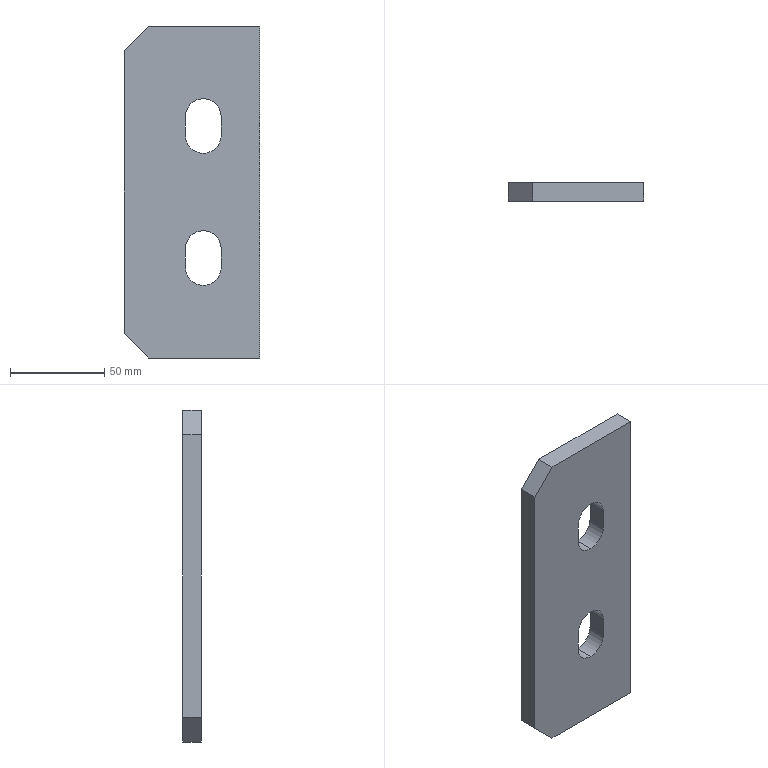Part | STEP file | 立柱填充筋Plate-194×150-2 | 1 solid | 18 faces | box 72 x 10 x 176 mm | volume 115559 mm3 | plane 12 | cylinder 6 | commonest cylinder face diameters 19 x6
STEP:
#1=CARTESIAN_POINT('',(0.,0.,0.));
#2=DIRECTION('',(0.,0.,1.));
#3=DIRECTION('',(1.,0.,0.));
#4=AXIS2_PLACEMENT_3D('',#1,#2,#3);
#5=CARTESIAN_POINT('',(51.5,0.,30.));
#6=VERTEX_POINT('',#5);
#7=CARTESIAN_POINT('',(51.5,10.,30.));
#8=VERTEX_POINT('',#7);
#9=CARTESIAN_POINT('',(51.5,40.,30.));
#10=DIRECTION('',(0.,1.,0.));
#11=VECTOR('',#10,1.);
#12=LINE('',#9,#11);
#13=CARTESIAN_POINT('',(42.,0.,30.));
#14=DIRECTION('',(0.,-1.,0.));
#15=DIRECTION('',(0.,0.,-1.));
#16=AXIS2_PLACEMENT_3D('',#13,#14,#15);
#17=CYLINDRICAL_SURFACE('',#16,9.5);
#18=CARTESIAN_POINT('',(1.571,-40.));
#19=DIRECTION('',(0.,-1.));
#20=VECTOR('',#19,1.);
#21=LINE('',#18,#20);
#22=(GEOMETRIC_REPRESENTATION_CONTEXT(2)PARAMETRIC_REPRESENTATION_CONTEXT()REPRESENTATION_CONTEXT('',''));
#23=DEFINITIONAL_REPRESENTATION('',(#21),#22);
#24=PCURVE('',#17,#23);
#25=CARTESIAN_POINT('',(51.5,40.,40.));
#26=DIRECTION('',(-1.,0.,0.));
#27=DIRECTION('',(0.,-1.,0.));
#28=AXIS2_PLACEMENT_3D('',#25,#26,#27);
#29=PLANE('',#28);
#30=CARTESIAN_POINT('',(0.,-10.));
#31=DIRECTION('',(-1.,0.));
#32=VECTOR('',#31,1.);
#33=LINE('',#30,#32);
#34=(GEOMETRIC_REPRESENTATION_CONTEXT(2)PARAMETRIC_REPRESENTATION_CONTEXT()REPRESENTATION_CONTEXT('',''));
#35=DEFINITIONAL_REPRESENTATION('',(#33),#34);
#36=PCURVE('',#29,#35);
#37=SURFACE_CURVE('',#12,(#24,#36),.PCURVE_S1.);
#38=EDGE_CURVE('',#6,#8,#37,.T.);
#39=ORIENTED_EDGE('',*,*,#38,.F.);
#40=CARTESIAN_POINT('',(42.,0.,20.5));
#41=VERTEX_POINT('',#40);
#42=CARTESIAN_POINT('',(42.,0.,30.));
#43=DIRECTION('',(0.,-1.,0.));
#44=DIRECTION('',(0.,0.,-1.));
#45=AXIS2_PLACEMENT_3D('',#42,#43,#44);
#46=CIRCLE('',#45,9.5);
#47=CARTESIAN_POINT('',(0.,0.));
#48=DIRECTION('',(1.,0.));
#49=VECTOR('',#48,1.);
#50=LINE('',#47,#49);
#51=(GEOMETRIC_REPRESENTATION_CONTEXT(2)PARAMETRIC_REPRESENTATION_CONTEXT()REPRESENTATION_CONTEXT('',''));
#52=DEFINITIONAL_REPRESENTATION('',(#50),#51);
#53=PCURVE('',#17,#52);
#54=CARTESIAN_POINT('',(0.,0.,0.));
#55=DIRECTION('',(0.,-1.,0.));
#56=DIRECTION('',(0.,0.,-1.));
#57=AXIS2_PLACEMENT_3D('',#54,#55,#56);
#58=PLANE('',#57);
#59=CARTESIAN_POINT('',(-30.,42.));
#60=DIRECTION('',(1.,0.));
#61=AXIS2_PLACEMENT_2D('',#59,#60);
#62=CIRCLE('',#61,9.5);
#63=(GEOMETRIC_REPRESENTATION_CONTEXT(2)PARAMETRIC_REPRESENTATION_CONTEXT()REPRESENTATION_CONTEXT('',''));
#64=DEFINITIONAL_REPRESENTATION('',(#62),#63);
#65=PCURVE('',#58,#64);
#66=SURFACE_CURVE('',#46,(#53,#65),.PCURVE_S1.);
#67=EDGE_CURVE('',#41,#6,#66,.T.);
#68=ORIENTED_EDGE('',*,*,#67,.F.);
#69=CARTESIAN_POINT('',(42.,10.,20.5));
#70=VERTEX_POINT('',#69);
#71=CARTESIAN_POINT('',(42.,0.,20.5));
#72=DIRECTION('',(0.,-1.,0.));
#73=VECTOR('',#72,1.);
#74=LINE('',#71,#73);
#75=CARTESIAN_POINT('',(0.,0.));
#76=DIRECTION('',(0.,1.));
#77=VECTOR('',#76,1.);
#78=LINE('',#75,#77);
#79=(GEOMETRIC_REPRESENTATION_CONTEXT(2)PARAMETRIC_REPRESENTATION_CONTEXT()REPRESENTATION_CONTEXT('',''));
#80=DEFINITIONAL_REPRESENTATION('',(#78),#79);
#81=PCURVE('',#17,#80);
#82=CARTESIAN_POINT('',(42.,0.,30.));
#83=DIRECTION('',(0.,-1.,0.));
#84=DIRECTION('',(0.,0.,-1.));
#85=AXIS2_PLACEMENT_3D('',#82,#83,#84);
#86=CYLINDRICAL_SURFACE('',#85,9.5);
#87=CARTESIAN_POINT('',(6.283,0.));
#88=DIRECTION('',(0.,1.));
#89=VECTOR('',#88,1.);
#90=LINE('',#87,#89);
#91=(GEOMETRIC_REPRESENTATION_CONTEXT(2)PARAMETRIC_REPRESENTATION_CONTEXT()REPRESENTATION_CONTEXT('',''));
#92=DEFINITIONAL_REPRESENTATION('',(#90),#91);
#93=PCURVE('',#86,#92);
#94=SURFACE_CURVE('',#74,(#81,#93),.PCURVE_S1.);
#95=EDGE_CURVE('',#70,#41,#94,.T.);
#96=ORIENTED_EDGE('',*,*,#95,.F.);
#97=CARTESIAN_POINT('',(42.,10.,30.));
#98=DIRECTION('',(0.,-1.,0.));
#99=DIRECTION('',(0.,0.,-1.));
#100=AXIS2_PLACEMENT_3D('',#97,#98,#99);
#101=CIRCLE('',#100,9.5);
#102=CARTESIAN_POINT('',(0.,-10.));
#103=DIRECTION('',(1.,0.));
#104=VECTOR('',#103,1.);
#105=LINE('',#102,#104);
#106=(GEOMETRIC_REPRESENTATION_CONTEXT(2)PARAMETRIC_REPRESENTATION_CONTEXT()REPRESENTATION_CONTEXT('',''));
#107=DEFINITIONAL_REPRESENTATION('',(#105),#106);
#108=PCURVE('',#17,#107);
#109=CARTESIAN_POINT('',(0.,10.,0.));
#110=DIRECTION('',(0.,-1.,0.));
#111=DIRECTION('',(0.,0.,-1.));
#112=AXIS2_PLACEMENT_3D('',#109,#110,#111);
#113=PLANE('',#112);
#114=CARTESIAN_POINT('',(-30.,42.));
#115=DIRECTION('',(1.,0.));
#116=AXIS2_PLACEMENT_2D('',#114,#115);
#117=CIRCLE('',#116,9.5);
#118=(GEOMETRIC_REPRESENTATION_CONTEXT(2)PARAMETRIC_REPRESENTATION_CONTEXT()REPRESENTATION_CONTEXT('',''));
#119=DEFINITIONAL_REPRESENTATION('',(#117),#118);
#120=PCURVE('',#113,#119);
#121=SURFACE_CURVE('',#101,(#108,#120),.PCURVE_S1.);
#122=EDGE_CURVE('',#70,#8,#121,.T.);
#123=ORIENTED_EDGE('',*,*,#122,.T.);
#124=EDGE_LOOP('',(#39,#68,#96,#123));
#125=FACE_BOUND('',#124,.F.);
#126=ADVANCED_FACE('',(#125),#17,.F.);
#127=CARTESIAN_POINT('',(51.5,0.,-40.));
#128=VERTEX_POINT('',#127);
#129=CARTESIAN_POINT('',(51.5,10.,-40.));
#130=VERTEX_POINT('',#129);
#131=CARTESIAN_POINT('',(51.5,40.,-40.));
#132=DIRECTION('',(0.,1.,0.));
#133=VECTOR('',#132,1.);
#134=LINE('',#131,#133);
#135=CARTESIAN_POINT('',(42.,0.,-40.));
#136=DIRECTION('',(0.,-1.,0.));
#137=DIRECTION('',(0.,0.,-1.));
#138=AXIS2_PLACEMENT_3D('',#135,#136,#137);
#139=CYLINDRICAL_SURFACE('',#138,9.5);
#140=CARTESIAN_POINT('',(1.571,-40.));
#141=DIRECTION('',(0.,-1.));
#142=VECTOR('',#141,1.);
#143=LINE('',#140,#142);
#144=(GEOMETRIC_REPRESENTATION_CONTEXT(2)PARAMETRIC_REPRESENTATION_CONTEXT()REPRESENTATION_CONTEXT('',''));
#145=DEFINITIONAL_REPRESENTATION('',(#143),#144);
#146=PCURVE('',#139,#145);
#147=CARTESIAN_POINT('',(51.5,40.,-30.));
#148=DIRECTION('',(-1.,0.,0.));
#149=DIRECTION('',(0.,-1.,0.));
#150=AXIS2_PLACEMENT_3D('',#147,#148,#149);
#151=PLANE('',#150);
#152=CARTESIAN_POINT('',(0.,-10.));
#153=DIRECTION('',(-1.,0.));
#154=VECTOR('',#153,1.);
#155=LINE('',#152,#154);
#156=(GEOMETRIC_REPRESENTATION_CONTEXT(2)PARAMETRIC_REPRESENTATION_CONTEXT()REPRESENTATION_CONTEXT('',''));
#157=DEFINITIONAL_REPRESENTATION('',(#155),#156);
#158=PCURVE('',#151,#157);
#159=SURFACE_CURVE('',#134,(#146,#158),.PCURVE_S1.);
#160=EDGE_CURVE('',#128,#130,#159,.T.);
#161=ORIENTED_EDGE('',*,*,#160,.F.);
#162=CARTESIAN_POINT('',(42.,0.,-49.5));
#163=VERTEX_POINT('',#162);
#164=CARTESIAN_POINT('',(42.,0.,-40.));
#165=DIRECTION('',(0.,-1.,0.));
#166=DIRECTION('',(0.,0.,-1.));
#167=AXIS2_PLACEMENT_3D('',#164,#165,#166);
#168=CIRCLE('',#167,9.5);
#169=CARTESIAN_POINT('',(0.,0.));
#170=DIRECTION('',(1.,0.));
#171=VECTOR('',#170,1.);
#172=LINE('',#169,#171);
#173=(GEOMETRIC_REPRESENTATION_CONTEXT(2)PARAMETRIC_REPRESENTATION_CONTEXT()REPRESENTATION_CONTEXT('',''));
#174=DEFINITIONAL_REPRESENTATION('',(#172),#173);
#175=PCURVE('',#139,#174);
#176=CARTESIAN_POINT('',(40.,42.));
#177=DIRECTION('',(1.,0.));
#178=AXIS2_PLACEMENT_2D('',#176,#177);
#179=CIRCLE('',#178,9.5);
#180=(GEOMETRIC_REPRESENTATION_CONTEXT(2)PARAMETRIC_REPRESENTATION_CONTEXT()REPRESENTATION_CONTEXT('',''));
#181=DEFINITIONAL_REPRESENTATION('',(#179),#180);
#182=PCURVE('',#58,#181);
#183=SURFACE_CURVE('',#168,(#175,#182),.PCURVE_S1.);
#184=EDGE_CURVE('',#163,#128,#183,.T.);
#185=ORIENTED_EDGE('',*,*,#184,.F.);
#186=CARTESIAN_POINT('',(42.,10.,-49.5));
#187=VERTEX_POINT('',#186);
#188=CARTESIAN_POINT('',(42.,0.,-49.5));
#189=DIRECTION('',(0.,-1.,0.));
#190=VECTOR('',#189,1.);
#191=LINE('',#188,#190);
#192=CARTESIAN_POINT('',(0.,0.));
#193=DIRECTION('',(0.,1.));
#194=VECTOR('',#193,1.);
#195=LINE('',#192,#194);
#196=(GEOMETRIC_REPRESENTATION_CONTEXT(2)PARAMETRIC_REPRESENTATION_CONTEXT()REPRESENTATION_CONTEXT('',''));
#197=DEFINITIONAL_REPRESENTATION('',(#195),#196);
#198=PCURVE('',#139,#197);
#199=CARTESIAN_POINT('',(42.,0.,-40.));
#200=DIRECTION('',(0.,-1.,0.));
#201=DIRECTION('',(0.,0.,-1.));
#202=AXIS2_PLACEMENT_3D('',#199,#200,#201);
#203=CYLINDRICAL_SURFACE('',#202,9.5);
#204=CARTESIAN_POINT('',(6.283,0.));
#205=DIRECTION('',(0.,1.));
#206=VECTOR('',#205,1.);
#207=LINE('',#204,#206);
#208=(GEOMETRIC_REPRESENTATION_CONTEXT(2)PARAMETRIC_REPRESENTATION_CONTEXT()REPRESENTATION_CONTEXT('',''));
#209=DEFINITIONAL_REPRESENTATION('',(#207),#208);
#210=PCURVE('',#203,#209);
#211=SURFACE_CURVE('',#191,(#198,#210),.PCURVE_S1.);
#212=EDGE_CURVE('',#187,#163,#211,.T.);
#213=ORIENTED_EDGE('',*,*,#212,.F.);
#214=CARTESIAN_POINT('',(42.,10.,-40.));
#215=DIRECTION('',(0.,-1.,0.));
#216=DIRECTION('',(0.,0.,-1.));
#217=AXIS2_PLACEMENT_3D('',#214,#215,#216);
#218=CIRCLE('',#217,9.5);
#219=CARTESIAN_POINT('',(0.,-10.));
#220=DIRECTION('',(1.,0.));
#221=VECTOR('',#220,1.);
#222=LINE('',#219,#221);
#223=(GEOMETRIC_REPRESENTATION_CONTEXT(2)PARAMETRIC_REPRESENTATION_CONTEXT()REPRESENTATION_CONTEXT('',''));
#224=DEFINITIONAL_REPRESENTATION('',(#222),#223);
#225=PCURVE('',#139,#224);
#226=CARTESIAN_POINT('',(40.,42.));
#227=DIRECTION('',(1.,0.));
#228=AXIS2_PLACEMENT_2D('',#226,#227);
#229=CIRCLE('',#228,9.5);
#230=(GEOMETRIC_REPRESENTATION_CONTEXT(2)PARAMETRIC_REPRESENTATION_CONTEXT()REPRESENTATION_CONTEXT('',''));
#231=DEFINITIONAL_REPRESENTATION('',(#229),#230);
#232=PCURVE('',#113,#231);
#233=SURFACE_CURVE('',#218,(#225,#232),.PCURVE_S1.);
#234=EDGE_CURVE('',#187,#130,#233,.T.);
#235=ORIENTED_EDGE('',*,*,#234,.T.);
#236=EDGE_LOOP('',(#161,#185,#213,#235));
#237=FACE_BOUND('',#236,.F.);
#238=ADVANCED_FACE('',(#237),#139,.F.);
#239=CARTESIAN_POINT('',(51.5,10.,40.));
#240=VERTEX_POINT('',#239);
#241=CARTESIAN_POINT('',(51.5,10.,0.));
#242=DIRECTION('',(0.,0.,-1.));
#243=VECTOR('',#242,1.);
#244=LINE('',#241,#243);
#245=CARTESIAN_POINT('',(0.,51.5));
#246=DIRECTION('',(1.,0.));
#247=VECTOR('',#246,1.);
#248=LINE('',#245,#247);
#249=(GEOMETRIC_REPRESENTATION_CONTEXT(2)PARAMETRIC_REPRESENTATION_CONTEXT()REPRESENTATION_CONTEXT('',''));
#250=DEFINITIONAL_REPRESENTATION('',(#248),#249);
#251=PCURVE('',#113,#250);
#252=CARTESIAN_POINT('',(30.,-40.));
#253=DIRECTION('',(0.,-1.));
#254=VECTOR('',#253,1.);
#255=LINE('',#252,#254);
#256=(GEOMETRIC_REPRESENTATION_CONTEXT(2)PARAMETRIC_REPRESENTATION_CONTEXT()REPRESENTATION_CONTEXT('',''));
#257=DEFINITIONAL_REPRESENTATION('',(#255),#256);
#258=PCURVE('',#29,#257);
#259=SURFACE_CURVE('',#244,(#251,#258),.PCURVE_S1.);
#260=EDGE_CURVE('',#240,#8,#259,.T.);
#261=ORIENTED_EDGE('',*,*,#260,.F.);
#262=CARTESIAN_POINT('',(32.5,10.,40.));
#263=VERTEX_POINT('',#262);
#264=CARTESIAN_POINT('',(42.,10.,40.));
#265=DIRECTION('',(0.,-1.,0.));
#266=DIRECTION('',(0.,0.,-1.));
#267=AXIS2_PLACEMENT_3D('',#264,#265,#266);
#268=CIRCLE('',#267,9.5);
#269=CARTESIAN_POINT('',(-40.,42.));
#270=DIRECTION('',(1.,0.));
#271=AXIS2_PLACEMENT_2D('',#269,#270);
#272=CIRCLE('',#271,9.5);
#273=(GEOMETRIC_REPRESENTATION_CONTEXT(2)PARAMETRIC_REPRESENTATION_CONTEXT()REPRESENTATION_CONTEXT('',''));
#274=DEFINITIONAL_REPRESENTATION('',(#272),#273);
#275=PCURVE('',#113,#274);
#276=CARTESIAN_POINT('',(42.,0.,40.));
#277=DIRECTION('',(0.,-1.,0.));
#278=DIRECTION('',(0.,0.,-1.));
#279=AXIS2_PLACEMENT_3D('',#276,#277,#278);
#280=CYLINDRICAL_SURFACE('',#279,9.5);
#281=CARTESIAN_POINT('',(0.,-10.));
#282=DIRECTION('',(1.,0.));
#283=VECTOR('',#282,1.);
#284=LINE('',#281,#283);
#285=(GEOMETRIC_REPRESENTATION_CONTEXT(2)PARAMETRIC_REPRESENTATION_CONTEXT()REPRESENTATION_CONTEXT('',''));
#286=DEFINITIONAL_REPRESENTATION('',(#284),#285);
#287=PCURVE('',#280,#286);
#288=SURFACE_CURVE('',#268,(#275,#287),.PCURVE_S1.);
#289=EDGE_CURVE('',#240,#263,#288,.T.);
#290=ORIENTED_EDGE('',*,*,#289,.T.);
#291=CARTESIAN_POINT('',(32.5,10.,30.));
#292=VERTEX_POINT('',#291);
#293=CARTESIAN_POINT('',(32.5,10.,0.));
#294=DIRECTION('',(0.,0.,-1.));
#295=VECTOR('',#294,1.);
#296=LINE('',#293,#295);
#297=CARTESIAN_POINT('',(0.,32.5));
#298=DIRECTION('',(1.,0.));
#299=VECTOR('',#298,1.);
#300=LINE('',#297,#299);
#301=(GEOMETRIC_REPRESENTATION_CONTEXT(2)PARAMETRIC_REPRESENTATION_CONTEXT()REPRESENTATION_CONTEXT('',''));
#302=DEFINITIONAL_REPRESENTATION('',(#300),#301);
#303=PCURVE('',#113,#302);
#304=CARTESIAN_POINT('',(32.5,0.,40.));
#305=DIRECTION('',(-1.,0.,0.));
#306=DIRECTION('',(0.,0.,1.));
#307=AXIS2_PLACEMENT_3D('',#304,#305,#306);
#308=PLANE('',#307);
#309=CARTESIAN_POINT('',(-40.,10.));
#310=DIRECTION('',(-1.,0.));
#311=VECTOR('',#310,1.);
#312=LINE('',#309,#311);
#313=(GEOMETRIC_REPRESENTATION_CONTEXT(2)PARAMETRIC_REPRESENTATION_CONTEXT()REPRESENTATION_CONTEXT('',''));
#314=DEFINITIONAL_REPRESENTATION('',(#312),#313);
#315=PCURVE('',#308,#314);
#316=SURFACE_CURVE('',#296,(#303,#315),.PCURVE_S1.);
#317=EDGE_CURVE('',#263,#292,#316,.T.);
#318=ORIENTED_EDGE('',*,*,#317,.T.);
#319=CARTESIAN_POINT('',(42.,10.,30.));
#320=DIRECTION('',(0.,-1.,0.));
#321=DIRECTION('',(0.,0.,-1.));
#322=AXIS2_PLACEMENT_3D('',#319,#320,#321);
#323=CIRCLE('',#322,9.5);
#324=CARTESIAN_POINT('',(-30.,42.));
#325=DIRECTION('',(1.,0.));
#326=AXIS2_PLACEMENT_2D('',#324,#325);
#327=CIRCLE('',#326,9.5);
#328=(GEOMETRIC_REPRESENTATION_CONTEXT(2)PARAMETRIC_REPRESENTATION_CONTEXT()REPRESENTATION_CONTEXT('',''));
#329=DEFINITIONAL_REPRESENTATION('',(#327),#328);
#330=PCURVE('',#113,#329);
#331=CARTESIAN_POINT('',(0.,-10.));
#332=DIRECTION('',(1.,0.));
#333=VECTOR('',#332,1.);
#334=LINE('',#331,#333);
#335=(GEOMETRIC_REPRESENTATION_CONTEXT(2)PARAMETRIC_REPRESENTATION_CONTEXT()REPRESENTATION_CONTEXT('',''));
#336=DEFINITIONAL_REPRESENTATION('',(#334),#335);
#337=PCURVE('',#86,#336);
#338=SURFACE_CURVE('',#323,(#330,#337),.PCURVE_S1.);
#339=EDGE_CURVE('',#292,#70,#338,.T.);
#340=ORIENTED_EDGE('',*,*,#339,.T.);
#341=ORIENTED_EDGE('',*,*,#122,.T.);
#342=EDGE_LOOP('',(#261,#290,#318,#340,#341));
#343=FACE_BOUND('',#342,.T.);
#344=CARTESIAN_POINT('',(0.,10.,-75.));
#345=VERTEX_POINT('',#344);
#346=CARTESIAN_POINT('',(0.,10.,75.));
#347=VERTEX_POINT('',#346);
#348=CARTESIAN_POINT('',(0.,10.,88.));
#349=DIRECTION('',(0.,0.,1.));
#350=VECTOR('',#349,1.);
#351=LINE('',#348,#350);
#352=CARTESIAN_POINT('',(-88.,0.));
#353=DIRECTION('',(-1.,0.));
#354=VECTOR('',#353,1.);
#355=LINE('',#352,#354);
#356=(GEOMETRIC_REPRESENTATION_CONTEXT(2)PARAMETRIC_REPRESENTATION_CONTEXT()REPRESENTATION_CONTEXT('',''));
#357=DEFINITIONAL_REPRESENTATION('',(#355),#356);
#358=PCURVE('',#113,#357);
#359=CARTESIAN_POINT('',(0.,10.,88.));
#360=DIRECTION('',(1.,0.,0.));
#361=DIRECTION('',(0.,0.,-1.));
#362=AXIS2_PLACEMENT_3D('',#359,#360,#361);
#363=PLANE('',#362);
#364=CARTESIAN_POINT('',(0.,0.));
#365=DIRECTION('',(-1.,0.));
#366=VECTOR('',#365,1.);
#367=LINE('',#364,#366);
#368=(GEOMETRIC_REPRESENTATION_CONTEXT(2)PARAMETRIC_REPRESENTATION_CONTEXT()REPRESENTATION_CONTEXT('',''));
#369=DEFINITIONAL_REPRESENTATION('',(#367),#368);
#370=PCURVE('',#363,#369);
#371=SURFACE_CURVE('',#351,(#358,#370),.PCURVE_S1.);
#372=EDGE_CURVE('',#345,#347,#371,.T.);
#373=ORIENTED_EDGE('',*,*,#372,.T.);
#374=CARTESIAN_POINT('',(13.,10.,88.));
#375=VERTEX_POINT('',#374);
#376=CARTESIAN_POINT('',(13.,10.,88.));
#377=DIRECTION('',(0.7071,0.,0.7071));
#378=VECTOR('',#377,1.);
#379=LINE('',#376,#378);
#380=CARTESIAN_POINT('',(-88.,13.));
#381=DIRECTION('',(-0.7071,0.7071));
#382=VECTOR('',#381,1.);
#383=LINE('',#380,#382);
#384=(GEOMETRIC_REPRESENTATION_CONTEXT(2)PARAMETRIC_REPRESENTATION_CONTEXT()REPRESENTATION_CONTEXT('',''));
#385=DEFINITIONAL_REPRESENTATION('',(#383),#384);
#386=PCURVE('',#113,#385);
#387=CARTESIAN_POINT('',(13.,10.,88.));
#388=DIRECTION('',(0.7071,0.,-0.7071));
#389=DIRECTION('',(0.,-1.,0.));
#390=AXIS2_PLACEMENT_3D('',#387,#388,#389);
#391=PLANE('',#390);
#392=CARTESIAN_POINT('',(0.,0.));
#393=DIRECTION('',(0.,-1.));
#394=VECTOR('',#393,1.);
#395=LINE('',#392,#394);
#396=(GEOMETRIC_REPRESENTATION_CONTEXT(2)PARAMETRIC_REPRESENTATION_CONTEXT()REPRESENTATION_CONTEXT('',''));
#397=DEFINITIONAL_REPRESENTATION('',(#395),#396);
#398=PCURVE('',#391,#397);
#399=SURFACE_CURVE('',#379,(#386,#398),.PCURVE_S1.);
#400=EDGE_CURVE('',#347,#375,#399,.T.);
#401=ORIENTED_EDGE('',*,*,#400,.T.);
#402=CARTESIAN_POINT('',(72.,10.,88.));
#403=VERTEX_POINT('',#402);
#404=CARTESIAN_POINT('',(72.,10.,88.));
#405=DIRECTION('',(1.,0.,0.));
#406=VECTOR('',#405,1.);
#407=LINE('',#404,#406);
#408=CARTESIAN_POINT('',(-88.,72.));
#409=DIRECTION('',(0.,1.));
#410=VECTOR('',#409,1.);
#411=LINE('',#408,#410);
#412=(GEOMETRIC_REPRESENTATION_CONTEXT(2)PARAMETRIC_REPRESENTATION_CONTEXT()REPRESENTATION_CONTEXT('',''));
#413=DEFINITIONAL_REPRESENTATION('',(#411),#412);
#414=PCURVE('',#113,#413);
#415=CARTESIAN_POINT('',(72.,10.,88.));
#416=DIRECTION('',(0.,0.,-1.));
#417=DIRECTION('',(-1.,0.,0.));
#418=AXIS2_PLACEMENT_3D('',#415,#416,#417);
#419=PLANE('',#418);
#420=CARTESIAN_POINT('',(0.,0.));
#421=DIRECTION('',(-1.,0.));
#422=VECTOR('',#421,1.);
#423=LINE('',#420,#422);
#424=(GEOMETRIC_REPRESENTATION_CONTEXT(2)PARAMETRIC_REPRESENTATION_CONTEXT()REPRESENTATION_CONTEXT('',''));
#425=DEFINITIONAL_REPRESENTATION('',(#423),#424);
#426=PCURVE('',#419,#425);
#427=SURFACE_CURVE('',#407,(#414,#426),.PCURVE_S1.);
#428=EDGE_CURVE('',#375,#403,#427,.T.);
#429=ORIENTED_EDGE('',*,*,#428,.T.);
#430=CARTESIAN_POINT('',(72.,10.,-88.));
#431=VERTEX_POINT('',#430);
#432=CARTESIAN_POINT('',(72.,10.,-88.));
#433=DIRECTION('',(0.,0.,-1.));
#434=VECTOR('',#433,1.);
#435=LINE('',#432,#434);
#436=CARTESIAN_POINT('',(88.,72.));
#437=DIRECTION('',(1.,0.));
#438=VECTOR('',#437,1.);
#439=LINE('',#436,#438);
#440=(GEOMETRIC_REPRESENTATION_CONTEXT(2)PARAMETRIC_REPRESENTATION_CONTEXT()REPRESENTATION_CONTEXT('',''));
#441=DEFINITIONAL_REPRESENTATION('',(#439),#440);
#442=PCURVE('',#113,#441);
#443=CARTESIAN_POINT('',(72.,10.,-88.));
#444=DIRECTION('',(-1.,0.,0.));
#445=DIRECTION('',(0.,0.,1.));
#446=AXIS2_PLACEMENT_3D('',#443,#444,#445);
#447=PLANE('',#446);
#448=CARTESIAN_POINT('',(0.,0.));
#449=DIRECTION('',(-1.,0.));
#450=VECTOR('',#449,1.);
#451=LINE('',#448,#450);
#452=(GEOMETRIC_REPRESENTATION_CONTEXT(2)PARAMETRIC_REPRESENTATION_CONTEXT()REPRESENTATION_CONTEXT('',''));
#453=DEFINITIONAL_REPRESENTATION('',(#451),#452);
#454=PCURVE('',#447,#453);
#455=SURFACE_CURVE('',#435,(#442,#454),.PCURVE_S1.);
#456=EDGE_CURVE('',#403,#431,#455,.T.);
#457=ORIENTED_EDGE('',*,*,#456,.T.);
#458=CARTESIAN_POINT('',(13.,10.,-88.));
#459=VERTEX_POINT('',#458);
#460=CARTESIAN_POINT('',(0.,10.,-88.));
#461=DIRECTION('',(-1.,0.,0.));
#462=VECTOR('',#461,1.);
#463=LINE('',#460,#462);
#464=CARTESIAN_POINT('',(88.,0.));
#465=DIRECTION('',(0.,-1.));
#466=VECTOR('',#465,1.);
#467=LINE('',#464,#466);
#468=(GEOMETRIC_REPRESENTATION_CONTEXT(2)PARAMETRIC_REPRESENTATION_CONTEXT()REPRESENTATION_CONTEXT('',''));
#469=DEFINITIONAL_REPRESENTATION('',(#467),#468);
#470=PCURVE('',#113,#469);
#471=CARTESIAN_POINT('',(0.,10.,-88.));
#472=DIRECTION('',(0.,0.,1.));
#473=DIRECTION('',(1.,0.,0.));
#474=AXIS2_PLACEMENT_3D('',#471,#472,#473);
#475=PLANE('',#474);
#476=CARTESIAN_POINT('',(0.,0.));
#477=DIRECTION('',(-1.,0.));
#478=VECTOR('',#477,1.);
#479=LINE('',#476,#478);
#480=(GEOMETRIC_REPRESENTATION_CONTEXT(2)PARAMETRIC_REPRESENTATION_CONTEXT()REPRESENTATION_CONTEXT('',''));
#481=DEFINITIONAL_REPRESENTATION('',(#479),#480);
#482=PCURVE('',#475,#481);
#483=SURFACE_CURVE('',#463,(#470,#482),.PCURVE_S1.);
#484=EDGE_CURVE('',#431,#459,#483,.T.);
#485=ORIENTED_EDGE('',*,*,#484,.T.);
#486=CARTESIAN_POINT('',(0.,10.,-75.));
#487=DIRECTION('',(-0.7071,0.,0.7071));
#488=VECTOR('',#487,1.);
#489=LINE('',#486,#488);
#490=CARTESIAN_POINT('',(75.,0.));
#491=DIRECTION('',(-0.7071,-0.7071));
#492=VECTOR('',#491,1.);
#493=LINE('',#490,#492);
#494=(GEOMETRIC_REPRESENTATION_CONTEXT(2)PARAMETRIC_REPRESENTATION_CONTEXT()REPRESENTATION_CONTEXT('',''));
#495=DEFINITIONAL_REPRESENTATION('',(#493),#494);
#496=PCURVE('',#113,#495);
#497=CARTESIAN_POINT('',(0.,10.,-75.));
#498=DIRECTION('',(0.7071,0.,0.7071));
#499=DIRECTION('',(0.,-1.,0.));
#500=AXIS2_PLACEMENT_3D('',#497,#498,#499);
#501=PLANE('',#500);
#502=CARTESIAN_POINT('',(0.,0.));
#503=DIRECTION('',(0.,-1.));
#504=VECTOR('',#503,1.);
#505=LINE('',#502,#504);
#506=(GEOMETRIC_REPRESENTATION_CONTEXT(2)PARAMETRIC_REPRESENTATION_CONTEXT()REPRESENTATION_CONTEXT('',''));
#507=DEFINITIONAL_REPRESENTATION('',(#505),#506);
#508=PCURVE('',#501,#507);
#509=SURFACE_CURVE('',#489,(#496,#508),.PCURVE_S1.);
#510=EDGE_CURVE('',#459,#345,#509,.T.);
#511=ORIENTED_EDGE('',*,*,#510,.T.);
#512=EDGE_LOOP('',(#373,#401,#429,#457,#485,#511));
#513=FACE_BOUND('',#512,.T.);
#514=CARTESIAN_POINT('',(51.5,10.,-30.));
#515=VERTEX_POINT('',#514);
#516=CARTESIAN_POINT('',(51.5,10.,0.));
#517=DIRECTION('',(0.,0.,-1.));
#518=VECTOR('',#517,1.);
#519=LINE('',#516,#518);
#520=CARTESIAN_POINT('',(0.,51.5));
#521=DIRECTION('',(1.,0.));
#522=VECTOR('',#521,1.);
#523=LINE('',#520,#522);
#524=(GEOMETRIC_REPRESENTATION_CONTEXT(2)PARAMETRIC_REPRESENTATION_CONTEXT()REPRESENTATION_CONTEXT('',''));
#525=DEFINITIONAL_REPRESENTATION('',(#523),#524);
#526=PCURVE('',#113,#525);
#527=CARTESIAN_POINT('',(30.,30.));
#528=DIRECTION('',(0.,-1.));
#529=VECTOR('',#528,1.);
#530=LINE('',#527,#529);
#531=(GEOMETRIC_REPRESENTATION_CONTEXT(2)PARAMETRIC_REPRESENTATION_CONTEXT()REPRESENTATION_CONTEXT('',''));
#532=DEFINITIONAL_REPRESENTATION('',(#530),#531);
#533=PCURVE('',#151,#532);
#534=SURFACE_CURVE('',#519,(#526,#533),.PCURVE_S1.);
#535=EDGE_CURVE('',#515,#130,#534,.T.);
#536=ORIENTED_EDGE('',*,*,#535,.F.);
#537=CARTESIAN_POINT('',(32.5,10.,-30.));
#538=VERTEX_POINT('',#537);
#539=CARTESIAN_POINT('',(42.,10.,-30.));
#540=DIRECTION('',(0.,-1.,0.));
#541=DIRECTION('',(0.,0.,-1.));
#542=AXIS2_PLACEMENT_3D('',#539,#540,#541);
#543=CIRCLE('',#542,9.5);
#544=CARTESIAN_POINT('',(30.,42.));
#545=DIRECTION('',(1.,0.));
#546=AXIS2_PLACEMENT_2D('',#544,#545);
#547=CIRCLE('',#546,9.5);
#548=(GEOMETRIC_REPRESENTATION_CONTEXT(2)PARAMETRIC_REPRESENTATION_CONTEXT()REPRESENTATION_CONTEXT('',''));
#549=DEFINITIONAL_REPRESENTATION('',(#547),#548);
#550=PCURVE('',#113,#549);
#551=CARTESIAN_POINT('',(42.,0.,-30.));
#552=DIRECTION('',(0.,-1.,0.));
#553=DIRECTION('',(0.,0.,-1.));
#554=AXIS2_PLACEMENT_3D('',#551,#552,#553);
#555=CYLINDRICAL_SURFACE('',#554,9.5);
#556=CARTESIAN_POINT('',(0.,-10.));
#557=DIRECTION('',(1.,0.));
#558=VECTOR('',#557,1.);
#559=LINE('',#556,#558);
#560=(GEOMETRIC_REPRESENTATION_CONTEXT(2)PARAMETRIC_REPRESENTATION_CONTEXT()REPRESENTATION_CONTEXT('',''));
#561=DEFINITIONAL_REPRESENTATION('',(#559),#560);
#562=PCURVE('',#555,#561);
#563=SURFACE_CURVE('',#543,(#550,#562),.PCURVE_S1.);
#564=EDGE_CURVE('',#515,#538,#563,.T.);
#565=ORIENTED_EDGE('',*,*,#564,.T.);
#566=CARTESIAN_POINT('',(32.5,10.,-40.));
#567=VERTEX_POINT('',#566);
#568=CARTESIAN_POINT('',(32.5,10.,0.));
#569=DIRECTION('',(0.,0.,-1.));
#570=VECTOR('',#569,1.);
#571=LINE('',#568,#570);
#572=CARTESIAN_POINT('',(0.,32.5));
#573=DIRECTION('',(1.,0.));
#574=VECTOR('',#573,1.);
#575=LINE('',#572,#574);
#576=(GEOMETRIC_REPRESENTATION_CONTEXT(2)PARAMETRIC_REPRESENTATION_CONTEXT()REPRESENTATION_CONTEXT('',''));
#577=DEFINITIONAL_REPRESENTATION('',(#575),#576);
#578=PCURVE('',#113,#577);
#579=CARTESIAN_POINT('',(32.5,0.,-30.));
#580=DIRECTION('',(-1.,0.,0.));
#581=DIRECTION('',(0.,0.,1.));
#582=AXIS2_PLACEMENT_3D('',#579,#580,#581);
#583=PLANE('',#582);
#584=CARTESIAN_POINT('',(30.,10.));
#585=DIRECTION('',(-1.,0.));
#586=VECTOR('',#585,1.);
#587=LINE('',#584,#586);
#588=(GEOMETRIC_REPRESENTATION_CONTEXT(2)PARAMETRIC_REPRESENTATION_CONTEXT()REPRESENTATION_CONTEXT('',''));
#589=DEFINITIONAL_REPRESENTATION('',(#587),#588);
#590=PCURVE('',#583,#589);
#591=SURFACE_CURVE('',#571,(#578,#590),.PCURVE_S1.);
#592=EDGE_CURVE('',#538,#567,#591,.T.);
#593=ORIENTED_EDGE('',*,*,#592,.T.);
#594=CARTESIAN_POINT('',(42.,10.,-40.));
#595=DIRECTION('',(0.,-1.,0.));
#596=DIRECTION('',(0.,0.,-1.));
#597=AXIS2_PLACEMENT_3D('',#594,#595,#596);
#598=CIRCLE('',#597,9.5);
#599=CARTESIAN_POINT('',(40.,42.));
#600=DIRECTION('',(1.,0.));
#601=AXIS2_PLACEMENT_2D('',#599,#600);
#602=CIRCLE('',#601,9.5);
#603=(GEOMETRIC_REPRESENTATION_CONTEXT(2)PARAMETRIC_REPRESENTATION_CONTEXT()REPRESENTATION_CONTEXT('',''));
#604=DEFINITIONAL_REPRESENTATION('',(#602),#603);
#605=PCURVE('',#113,#604);
#606=CARTESIAN_POINT('',(0.,-10.));
#607=DIRECTION('',(1.,0.));
#608=VECTOR('',#607,1.);
#609=LINE('',#606,#608);
#610=(GEOMETRIC_REPRESENTATION_CONTEXT(2)PARAMETRIC_REPRESENTATION_CONTEXT()REPRESENTATION_CONTEXT('',''));
#611=DEFINITIONAL_REPRESENTATION('',(#609),#610);
#612=PCURVE('',#203,#611);
#613=SURFACE_CURVE('',#598,(#605,#612),.PCURVE_S1.);
#614=EDGE_CURVE('',#567,#187,#613,.T.);
#615=ORIENTED_EDGE('',*,*,#614,.T.);
#616=ORIENTED_EDGE('',*,*,#234,.T.);
#617=EDGE_LOOP('',(#536,#565,#593,#615,#616));
#618=FACE_BOUND('',#617,.T.);
#619=ADVANCED_FACE('',(#343,#513,#618),#113,.F.);
#620=CARTESIAN_POINT('',(32.5,0.,30.));
#621=VERTEX_POINT('',#620);
#622=CARTESIAN_POINT('',(42.,0.,30.));
#623=DIRECTION('',(0.,-1.,0.));
#624=DIRECTION('',(0.,0.,-1.));
#625=AXIS2_PLACEMENT_3D('',#622,#623,#624);
#626=CIRCLE('',#625,9.5);
#627=CARTESIAN_POINT('',(-30.,42.));
#628=DIRECTION('',(1.,0.));
#629=AXIS2_PLACEMENT_2D('',#627,#628);
#630=CIRCLE('',#629,9.5);
#631=(GEOMETRIC_REPRESENTATION_CONTEXT(2)PARAMETRIC_REPRESENTATION_CONTEXT()REPRESENTATION_CONTEXT('',''));
#632=DEFINITIONAL_REPRESENTATION('',(#630),#631);
#633=PCURVE('',#58,#632);
#634=CARTESIAN_POINT('',(0.,0.));
#635=DIRECTION('',(1.,0.));
#636=VECTOR('',#635,1.);
#637=LINE('',#634,#636);
#638=(GEOMETRIC_REPRESENTATION_CONTEXT(2)PARAMETRIC_REPRESENTATION_CONTEXT()REPRESENTATION_CONTEXT('',''));
#639=DEFINITIONAL_REPRESENTATION('',(#637),#638);
#640=PCURVE('',#86,#639);
#641=SURFACE_CURVE('',#626,(#633,#640),.PCURVE_S1.);
#642=EDGE_CURVE('',#621,#41,#641,.T.);
#643=ORIENTED_EDGE('',*,*,#642,.F.);
#644=CARTESIAN_POINT('',(32.5,0.,40.));
#645=VERTEX_POINT('',#644);
#646=CARTESIAN_POINT('',(32.5,0.,40.));
#647=DIRECTION('',(0.,0.,-1.));
#648=VECTOR('',#647,1.);
#649=LINE('',#646,#648);
#650=CARTESIAN_POINT('',(-40.,32.5));
#651=DIRECTION('',(1.,0.));
#652=VECTOR('',#651,1.);
#653=LINE('',#650,#652);
#654=(GEOMETRIC_REPRESENTATION_CONTEXT(2)PARAMETRIC_REPRESENTATION_CONTEXT()REPRESENTATION_CONTEXT('',''));
#655=DEFINITIONAL_REPRESENTATION('',(#653),#654);
#656=PCURVE('',#58,#655);
#657=CARTESIAN_POINT('',(0.,0.));
#658=DIRECTION('',(-1.,0.));
#659=VECTOR('',#658,1.);
#660=LINE('',#657,#659);
#661=(GEOMETRIC_REPRESENTATION_CONTEXT(2)PARAMETRIC_REPRESENTATION_CONTEXT()REPRESENTATION_CONTEXT('',''));
#662=DEFINITIONAL_REPRESENTATION('',(#660),#661);
#663=PCURVE('',#308,#662);
#664=SURFACE_CURVE('',#649,(#656,#663),.PCURVE_S1.);
#665=EDGE_CURVE('',#645,#621,#664,.T.);
#666=ORIENTED_EDGE('',*,*,#665,.F.);
#667=CARTESIAN_POINT('',(51.5,0.,40.));
#668=VERTEX_POINT('',#667);
#669=CARTESIAN_POINT('',(42.,0.,40.));
#670=DIRECTION('',(0.,-1.,0.));
#671=DIRECTION('',(0.,0.,-1.));
#672=AXIS2_PLACEMENT_3D('',#669,#670,#671);
#673=CIRCLE('',#672,9.5);
#674=CARTESIAN_POINT('',(-40.,42.));
#675=DIRECTION('',(1.,0.));
#676=AXIS2_PLACEMENT_2D('',#674,#675);
#677=CIRCLE('',#676,9.5);
#678=(GEOMETRIC_REPRESENTATION_CONTEXT(2)PARAMETRIC_REPRESENTATION_CONTEXT()REPRESENTATION_CONTEXT('',''));
#679=DEFINITIONAL_REPRESENTATION('',(#677),#678);
#680=PCURVE('',#58,#679);
#681=CARTESIAN_POINT('',(0.,0.));
#682=DIRECTION('',(1.,0.));
#683=VECTOR('',#682,1.);
#684=LINE('',#681,#683);
#685=(GEOMETRIC_REPRESENTATION_CONTEXT(2)PARAMETRIC_REPRESENTATION_CONTEXT()REPRESENTATION_CONTEXT('',''));
#686=DEFINITIONAL_REPRESENTATION('',(#684),#685);
#687=PCURVE('',#280,#686);
#688=SURFACE_CURVE('',#673,(#680,#687),.PCURVE_S1.);
#689=EDGE_CURVE('',#668,#645,#688,.T.);
#690=ORIENTED_EDGE('',*,*,#689,.F.);
#691=CARTESIAN_POINT('',(51.5,0.,40.));
#692=DIRECTION('',(0.,0.,-1.));
#693=VECTOR('',#692,1.);
#694=LINE('',#691,#693);
#695=CARTESIAN_POINT('',(-40.,51.5));
#696=DIRECTION('',(1.,0.));
#697=VECTOR('',#696,1.);
#698=LINE('',#695,#697);
#699=(GEOMETRIC_REPRESENTATION_CONTEXT(2)PARAMETRIC_REPRESENTATION_CONTEXT()REPRESENTATION_CONTEXT('',''));
#700=DEFINITIONAL_REPRESENTATION('',(#698),#699);
#701=PCURVE('',#58,#700);
#702=CARTESIAN_POINT('',(40.,0.));
#703=DIRECTION('',(0.,-1.));
#704=VECTOR('',#703,1.);
#705=LINE('',#702,#704);
#706=(GEOMETRIC_REPRESENTATION_CONTEXT(2)PARAMETRIC_REPRESENTATION_CONTEXT()REPRESENTATION_CONTEXT('',''));
#707=DEFINITIONAL_REPRESENTATION('',(#705),#706);
#708=PCURVE('',#29,#707);
#709=SURFACE_CURVE('',#694,(#701,#708),.PCURVE_S1.);
#710=EDGE_CURVE('',#668,#6,#709,.T.);
#711=ORIENTED_EDGE('',*,*,#710,.T.);
#712=ORIENTED_EDGE('',*,*,#67,.F.);
#713=EDGE_LOOP('',(#643,#666,#690,#711,#712));
#714=FACE_BOUND('',#713,.T.);
#715=CARTESIAN_POINT('',(13.,0.,88.));
#716=VERTEX_POINT('',#715);
#717=CARTESIAN_POINT('',(72.,0.,88.));
#718=VERTEX_POINT('',#717);
#719=CARTESIAN_POINT('',(72.,0.,88.));
#720=DIRECTION('',(1.,0.,0.));
#721=VECTOR('',#720,1.);
#722=LINE('',#719,#721);
#723=CARTESIAN_POINT('',(-88.,72.));
#724=DIRECTION('',(0.,1.));
#725=VECTOR('',#724,1.);
#726=LINE('',#723,#725);
#727=(GEOMETRIC_REPRESENTATION_CONTEXT(2)PARAMETRIC_REPRESENTATION_CONTEXT()REPRESENTATION_CONTEXT('',''));
#728=DEFINITIONAL_REPRESENTATION('',(#726),#727);
#729=PCURVE('',#58,#728);
#730=CARTESIAN_POINT('',(0.,-10.));
#731=DIRECTION('',(-1.,0.));
#732=VECTOR('',#731,1.);
#733=LINE('',#730,#732);
#734=(GEOMETRIC_REPRESENTATION_CONTEXT(2)PARAMETRIC_REPRESENTATION_CONTEXT()REPRESENTATION_CONTEXT('',''));
#735=DEFINITIONAL_REPRESENTATION('',(#733),#734);
#736=PCURVE('',#419,#735);
#737=SURFACE_CURVE('',#722,(#729,#736),.PCURVE_S1.);
#738=EDGE_CURVE('',#716,#718,#737,.T.);
#739=ORIENTED_EDGE('',*,*,#738,.F.);
#740=CARTESIAN_POINT('',(0.,0.,75.));
#741=VERTEX_POINT('',#740);
#742=CARTESIAN_POINT('',(-37.5,0.,37.5));
#743=DIRECTION('',(-0.7071,0.,-0.7071));
#744=VECTOR('',#743,1.);
#745=LINE('',#742,#744);
#746=CARTESIAN_POINT('',(-37.5,-37.5));
#747=DIRECTION('',(0.7071,-0.7071));
#748=VECTOR('',#747,1.);
#749=LINE('',#746,#748);
#750=(GEOMETRIC_REPRESENTATION_CONTEXT(2)PARAMETRIC_REPRESENTATION_CONTEXT()REPRESENTATION_CONTEXT('',''));
#751=DEFINITIONAL_REPRESENTATION('',(#749),#750);
#752=PCURVE('',#58,#751);
#753=CARTESIAN_POINT('',(10.,71.418));
#754=DIRECTION('',(0.,1.));
#755=VECTOR('',#754,1.);
#756=LINE('',#753,#755);
#757=(GEOMETRIC_REPRESENTATION_CONTEXT(2)PARAMETRIC_REPRESENTATION_CONTEXT()REPRESENTATION_CONTEXT('',''));
#758=DEFINITIONAL_REPRESENTATION('',(#756),#757);
#759=PCURVE('',#391,#758);
#760=SURFACE_CURVE('',#745,(#752,#759),.PCURVE_S1.);
#761=EDGE_CURVE('',#716,#741,#760,.T.);
#762=ORIENTED_EDGE('',*,*,#761,.T.);
#763=CARTESIAN_POINT('',(0.,0.,-75.));
#764=VERTEX_POINT('',#763);
#765=CARTESIAN_POINT('',(0.,0.,88.));
#766=DIRECTION('',(0.,0.,1.));
#767=VECTOR('',#766,1.);
#768=LINE('',#765,#767);
#769=CARTESIAN_POINT('',(-88.,0.));
#770=DIRECTION('',(-1.,0.));
#771=VECTOR('',#770,1.);
#772=LINE('',#769,#771);
#773=(GEOMETRIC_REPRESENTATION_CONTEXT(2)PARAMETRIC_REPRESENTATION_CONTEXT()REPRESENTATION_CONTEXT('',''));
#774=DEFINITIONAL_REPRESENTATION('',(#772),#773);
#775=PCURVE('',#58,#774);
#776=CARTESIAN_POINT('',(0.,-10.));
#777=DIRECTION('',(-1.,0.));
#778=VECTOR('',#777,1.);
#779=LINE('',#776,#778);
#780=(GEOMETRIC_REPRESENTATION_CONTEXT(2)PARAMETRIC_REPRESENTATION_CONTEXT()REPRESENTATION_CONTEXT('',''));
#781=DEFINITIONAL_REPRESENTATION('',(#779),#780);
#782=PCURVE('',#363,#781);
#783=SURFACE_CURVE('',#768,(#775,#782),.PCURVE_S1.);
#784=EDGE_CURVE('',#764,#741,#783,.T.);
#785=ORIENTED_EDGE('',*,*,#784,.F.);
#786=CARTESIAN_POINT('',(13.,0.,-88.));
#787=VERTEX_POINT('',#786);
#788=CARTESIAN_POINT('',(-37.5,0.,-37.5));
#789=DIRECTION('',(0.7071,0.,-0.7071));
#790=VECTOR('',#789,1.);
#791=LINE('',#788,#790);
#792=CARTESIAN_POINT('',(37.5,-37.5));
#793=DIRECTION('',(0.7071,0.7071));
#794=VECTOR('',#793,1.);
#795=LINE('',#792,#794);
#796=(GEOMETRIC_REPRESENTATION_CONTEXT(2)PARAMETRIC_REPRESENTATION_CONTEXT()REPRESENTATION_CONTEXT('',''));
#797=DEFINITIONAL_REPRESENTATION('',(#795),#796);
#798=PCURVE('',#58,#797);
#799=CARTESIAN_POINT('',(10.,-53.033));
#800=DIRECTION('',(0.,1.));
#801=VECTOR('',#800,1.);
#802=LINE('',#799,#801);
#803=(GEOMETRIC_REPRESENTATION_CONTEXT(2)PARAMETRIC_REPRESENTATION_CONTEXT()REPRESENTATION_CONTEXT('',''));
#804=DEFINITIONAL_REPRESENTATION('',(#802),#803);
#805=PCURVE('',#501,#804);
#806=SURFACE_CURVE('',#791,(#798,#805),.PCURVE_S1.);
#807=EDGE_CURVE('',#764,#787,#806,.T.);
#808=ORIENTED_EDGE('',*,*,#807,.T.);
#809=CARTESIAN_POINT('',(72.,0.,-88.));
#810=VERTEX_POINT('',#809);
#811=CARTESIAN_POINT('',(0.,0.,-88.));
#812=DIRECTION('',(-1.,0.,0.));
#813=VECTOR('',#812,1.);
#814=LINE('',#811,#813);
#815=CARTESIAN_POINT('',(88.,0.));
#816=DIRECTION('',(0.,-1.));
#817=VECTOR('',#816,1.);
#818=LINE('',#815,#817);
#819=(GEOMETRIC_REPRESENTATION_CONTEXT(2)PARAMETRIC_REPRESENTATION_CONTEXT()REPRESENTATION_CONTEXT('',''));
#820=DEFINITIONAL_REPRESENTATION('',(#818),#819);
#821=PCURVE('',#58,#820);
#822=CARTESIAN_POINT('',(0.,-10.));
#823=DIRECTION('',(-1.,0.));
#824=VECTOR('',#823,1.);
#825=LINE('',#822,#824);
#826=(GEOMETRIC_REPRESENTATION_CONTEXT(2)PARAMETRIC_REPRESENTATION_CONTEXT()REPRESENTATION_CONTEXT('',''));
#827=DEFINITIONAL_REPRESENTATION('',(#825),#826);
#828=PCURVE('',#475,#827);
#829=SURFACE_CURVE('',#814,(#821,#828),.PCURVE_S1.);
#830=EDGE_CURVE('',#810,#787,#829,.T.);
#831=ORIENTED_EDGE('',*,*,#830,.F.);
#832=CARTESIAN_POINT('',(72.,0.,-88.));
#833=DIRECTION('',(0.,0.,-1.));
#834=VECTOR('',#833,1.);
#835=LINE('',#832,#834);
#836=CARTESIAN_POINT('',(88.,72.));
#837=DIRECTION('',(1.,0.));
#838=VECTOR('',#837,1.);
#839=LINE('',#836,#838);
#840=(GEOMETRIC_REPRESENTATION_CONTEXT(2)PARAMETRIC_REPRESENTATION_CONTEXT()REPRESENTATION_CONTEXT('',''));
#841=DEFINITIONAL_REPRESENTATION('',(#839),#840);
#842=PCURVE('',#58,#841);
#843=CARTESIAN_POINT('',(0.,-10.));
#844=DIRECTION('',(-1.,0.));
#845=VECTOR('',#844,1.);
#846=LINE('',#843,#845);
#847=(GEOMETRIC_REPRESENTATION_CONTEXT(2)PARAMETRIC_REPRESENTATION_CONTEXT()REPRESENTATION_CONTEXT('',''));
#848=DEFINITIONAL_REPRESENTATION('',(#846),#847);
#849=PCURVE('',#447,#848);
#850=SURFACE_CURVE('',#835,(#842,#849),.PCURVE_S1.);
#851=EDGE_CURVE('',#718,#810,#850,.T.);
#852=ORIENTED_EDGE('',*,*,#851,.F.);
#853=EDGE_LOOP('',(#739,#762,#785,#808,#831,#852));
#854=FACE_BOUND('',#853,.T.);
#855=CARTESIAN_POINT('',(51.5,0.,-30.));
#856=VERTEX_POINT('',#855);
#857=CARTESIAN_POINT('',(32.5,0.,-30.));
#858=VERTEX_POINT('',#857);
#859=CARTESIAN_POINT('',(42.,0.,-30.));
#860=DIRECTION('',(0.,-1.,0.));
#861=DIRECTION('',(0.,0.,-1.));
#862=AXIS2_PLACEMENT_3D('',#859,#860,#861);
#863=CIRCLE('',#862,9.5);
#864=CARTESIAN_POINT('',(30.,42.));
#865=DIRECTION('',(1.,0.));
#866=AXIS2_PLACEMENT_2D('',#864,#865);
#867=CIRCLE('',#866,9.5);
#868=(GEOMETRIC_REPRESENTATION_CONTEXT(2)PARAMETRIC_REPRESENTATION_CONTEXT()REPRESENTATION_CONTEXT('',''));
#869=DEFINITIONAL_REPRESENTATION('',(#867),#868);
#870=PCURVE('',#58,#869);
#871=CARTESIAN_POINT('',(0.,0.));
#872=DIRECTION('',(1.,0.));
#873=VECTOR('',#872,1.);
#874=LINE('',#871,#873);
#875=(GEOMETRIC_REPRESENTATION_CONTEXT(2)PARAMETRIC_REPRESENTATION_CONTEXT()REPRESENTATION_CONTEXT('',''));
#876=DEFINITIONAL_REPRESENTATION('',(#874),#875);
#877=PCURVE('',#555,#876);
#878=SURFACE_CURVE('',#863,(#870,#877),.PCURVE_S1.);
#879=EDGE_CURVE('',#856,#858,#878,.T.);
#880=ORIENTED_EDGE('',*,*,#879,.F.);
#881=CARTESIAN_POINT('',(51.5,0.,-30.));
#882=DIRECTION('',(0.,0.,-1.));
#883=VECTOR('',#882,1.);
#884=LINE('',#881,#883);
#885=CARTESIAN_POINT('',(30.,51.5));
#886=DIRECTION('',(1.,0.));
#887=VECTOR('',#886,1.);
#888=LINE('',#885,#887);
#889=(GEOMETRIC_REPRESENTATION_CONTEXT(2)PARAMETRIC_REPRESENTATION_CONTEXT()REPRESENTATION_CONTEXT('',''));
#890=DEFINITIONAL_REPRESENTATION('',(#888),#889);
#891=PCURVE('',#58,#890);
#892=CARTESIAN_POINT('',(40.,0.));
#893=DIRECTION('',(0.,-1.));
#894=VECTOR('',#893,1.);
#895=LINE('',#892,#894);
#896=(GEOMETRIC_REPRESENTATION_CONTEXT(2)PARAMETRIC_REPRESENTATION_CONTEXT()REPRESENTATION_CONTEXT('',''));
#897=DEFINITIONAL_REPRESENTATION('',(#895),#896);
#898=PCURVE('',#151,#897);
#899=SURFACE_CURVE('',#884,(#891,#898),.PCURVE_S1.);
#900=EDGE_CURVE('',#856,#128,#899,.T.);
#901=ORIENTED_EDGE('',*,*,#900,.T.);
#902=ORIENTED_EDGE('',*,*,#184,.F.);
#903=CARTESIAN_POINT('',(32.5,0.,-40.));
#904=VERTEX_POINT('',#903);
#905=CARTESIAN_POINT('',(42.,0.,-40.));
#906=DIRECTION('',(0.,-1.,0.));
#907=DIRECTION('',(0.,0.,-1.));
#908=AXIS2_PLACEMENT_3D('',#905,#906,#907);
#909=CIRCLE('',#908,9.5);
#910=CARTESIAN_POINT('',(40.,42.));
#911=DIRECTION('',(1.,0.));
#912=AXIS2_PLACEMENT_2D('',#910,#911);
#913=CIRCLE('',#912,9.5);
#914=(GEOMETRIC_REPRESENTATION_CONTEXT(2)PARAMETRIC_REPRESENTATION_CONTEXT()REPRESENTATION_CONTEXT('',''));
#915=DEFINITIONAL_REPRESENTATION('',(#913),#914);
#916=PCURVE('',#58,#915);
#917=CARTESIAN_POINT('',(0.,0.));
#918=DIRECTION('',(1.,0.));
#919=VECTOR('',#918,1.);
#920=LINE('',#917,#919);
#921=(GEOMETRIC_REPRESENTATION_CONTEXT(2)PARAMETRIC_REPRESENTATION_CONTEXT()REPRESENTATION_CONTEXT('',''));
#922=DEFINITIONAL_REPRESENTATION('',(#920),#921);
#923=PCURVE('',#203,#922);
#924=SURFACE_CURVE('',#909,(#916,#923),.PCURVE_S1.);
#925=EDGE_CURVE('',#904,#163,#924,.T.);
#926=ORIENTED_EDGE('',*,*,#925,.F.);
#927=CARTESIAN_POINT('',(32.5,0.,-30.));
#928=DIRECTION('',(0.,0.,-1.));
#929=VECTOR('',#928,1.);
#930=LINE('',#927,#929);
#931=CARTESIAN_POINT('',(30.,32.5));
#932=DIRECTION('',(1.,0.));
#933=VECTOR('',#932,1.);
#934=LINE('',#931,#933);
#935=(GEOMETRIC_REPRESENTATION_CONTEXT(2)PARAMETRIC_REPRESENTATION_CONTEXT()REPRESENTATION_CONTEXT('',''));
#936=DEFINITIONAL_REPRESENTATION('',(#934),#935);
#937=PCURVE('',#58,#936);
#938=CARTESIAN_POINT('',(0.,0.));
#939=DIRECTION('',(-1.,0.));
#940=VECTOR('',#939,1.);
#941=LINE('',#938,#940);
#942=(GEOMETRIC_REPRESENTATION_CONTEXT(2)PARAMETRIC_REPRESENTATION_CONTEXT()REPRESENTATION_CONTEXT('',''));
#943=DEFINITIONAL_REPRESENTATION('',(#941),#942);
#944=PCURVE('',#583,#943);
#945=SURFACE_CURVE('',#930,(#937,#944),.PCURVE_S1.);
#946=EDGE_CURVE('',#858,#904,#945,.T.);
#947=ORIENTED_EDGE('',*,*,#946,.F.);
#948=EDGE_LOOP('',(#880,#901,#902,#926,#947));
#949=FACE_BOUND('',#948,.T.);
#950=ADVANCED_FACE('',(#714,#854,#949),#58,.T.);
#951=ORIENTED_EDGE('',*,*,#851,.T.);
#952=CARTESIAN_POINT('',(72.,10.,-88.));
#953=DIRECTION('',(0.,-1.,0.));
#954=VECTOR('',#953,1.);
#955=LINE('',#952,#954);
#956=CARTESIAN_POINT('',(0.,0.));
#957=DIRECTION('',(0.,-1.));
#958=VECTOR('',#957,1.);
#959=LINE('',#956,#958);
#960=(GEOMETRIC_REPRESENTATION_CONTEXT(2)PARAMETRIC_REPRESENTATION_CONTEXT()REPRESENTATION_CONTEXT('',''));
#961=DEFINITIONAL_REPRESENTATION('',(#959),#960);
#962=PCURVE('',#447,#961);
#963=CARTESIAN_POINT('',(72.,0.));
#964=DIRECTION('',(0.,-1.));
#965=VECTOR('',#964,1.);
#966=LINE('',#963,#965);
#967=(GEOMETRIC_REPRESENTATION_CONTEXT(2)PARAMETRIC_REPRESENTATION_CONTEXT()REPRESENTATION_CONTEXT('',''));
#968=DEFINITIONAL_REPRESENTATION('',(#966),#967);
#969=PCURVE('',#475,#968);
#970=SURFACE_CURVE('',#955,(#962,#969),.PCURVE_S1.);
#971=EDGE_CURVE('',#431,#810,#970,.T.);
#972=ORIENTED_EDGE('',*,*,#971,.F.);
#973=ORIENTED_EDGE('',*,*,#456,.F.);
#974=CARTESIAN_POINT('',(72.,10.,88.));
#975=DIRECTION('',(0.,-1.,0.));
#976=VECTOR('',#975,1.);
#977=LINE('',#974,#976);
#978=CARTESIAN_POINT('',(176.,0.));
#979=DIRECTION('',(0.,-1.));
#980=VECTOR('',#979,1.);
#981=LINE('',#978,#980);
#982=(GEOMETRIC_REPRESENTATION_CONTEXT(2)PARAMETRIC_REPRESENTATION_CONTEXT()REPRESENTATION_CONTEXT('',''));
#983=DEFINITIONAL_REPRESENTATION('',(#981),#982);
#984=PCURVE('',#447,#983);
#985=CARTESIAN_POINT('',(0.,0.));
#986=DIRECTION('',(0.,-1.));
#987=VECTOR('',#986,1.);
#988=LINE('',#985,#987);
#989=(GEOMETRIC_REPRESENTATION_CONTEXT(2)PARAMETRIC_REPRESENTATION_CONTEXT()REPRESENTATION_CONTEXT('',''));
#990=DEFINITIONAL_REPRESENTATION('',(#988),#989);
#991=PCURVE('',#419,#990);
#992=SURFACE_CURVE('',#977,(#984,#991),.PCURVE_S1.);
#993=EDGE_CURVE('',#403,#718,#992,.T.);
#994=ORIENTED_EDGE('',*,*,#993,.T.);
#995=EDGE_LOOP('',(#951,#972,#973,#994));
#996=FACE_BOUND('',#995,.T.);
#997=ADVANCED_FACE('',(#996),#447,.F.);
#998=ORIENTED_EDGE('',*,*,#830,.T.);
#999=CARTESIAN_POINT('',(13.,10.,-88.));
#1000=DIRECTION('',(0.,1.,0.));
#1001=VECTOR('',#1000,1.);
#1002=LINE('',#999,#1001);
#1003=CARTESIAN_POINT('',(13.,0.));
#1004=DIRECTION('',(0.,1.));
#1005=VECTOR('',#1004,1.);
#1006=LINE('',#1003,#1005);
#1007=(GEOMETRIC_REPRESENTATION_CONTEXT(2)PARAMETRIC_REPRESENTATION_CONTEXT()REPRESENTATION_CONTEXT('',''));
#1008=DEFINITIONAL_REPRESENTATION('',(#1006),#1007);
#1009=PCURVE('',#475,#1008);
#1010=CARTESIAN_POINT('',(0.,18.385));
#1011=DIRECTION('',(-1.,0.));
#1012=VECTOR('',#1011,1.);
#1013=LINE('',#1010,#1012);
#1014=(GEOMETRIC_REPRESENTATION_CONTEXT(2)PARAMETRIC_REPRESENTATION_CONTEXT()REPRESENTATION_CONTEXT('',''));
#1015=DEFINITIONAL_REPRESENTATION('',(#1013),#1014);
#1016=PCURVE('',#501,#1015);
#1017=SURFACE_CURVE('',#1002,(#1009,#1016),.PCURVE_S1.);
#1018=EDGE_CURVE('',#787,#459,#1017,.T.);
#1019=ORIENTED_EDGE('',*,*,#1018,.T.);
#1020=ORIENTED_EDGE('',*,*,#484,.F.);
#1021=ORIENTED_EDGE('',*,*,#971,.T.);
#1022=EDGE_LOOP('',(#998,#1019,#1020,#1021));
#1023=FACE_BOUND('',#1022,.T.);
#1024=ADVANCED_FACE('',(#1023),#475,.F.);
#1025=ORIENTED_EDGE('',*,*,#784,.T.);
#1026=CARTESIAN_POINT('',(0.,10.,75.));
#1027=DIRECTION('',(0.,1.,0.));
#1028=VECTOR('',#1027,1.);
#1029=LINE('',#1026,#1028);
#1030=CARTESIAN_POINT('',(13.,0.));
#1031=DIRECTION('',(0.,1.));
#1032=VECTOR('',#1031,1.);
#1033=LINE('',#1030,#1032);
#1034=(GEOMETRIC_REPRESENTATION_CONTEXT(2)PARAMETRIC_REPRESENTATION_CONTEXT()REPRESENTATION_CONTEXT('',''));
#1035=DEFINITIONAL_REPRESENTATION('',(#1033),#1034);
#1036=PCURVE('',#363,#1035);
#1037=CARTESIAN_POINT('',(0.,18.385));
#1038=DIRECTION('',(-1.,0.));
#1039=VECTOR('',#1038,1.);
#1040=LINE('',#1037,#1039);
#1041=(GEOMETRIC_REPRESENTATION_CONTEXT(2)PARAMETRIC_REPRESENTATION_CONTEXT()REPRESENTATION_CONTEXT('',''));
#1042=DEFINITIONAL_REPRESENTATION('',(#1040),#1041);
#1043=PCURVE('',#391,#1042);
#1044=SURFACE_CURVE('',#1029,(#1036,#1043),.PCURVE_S1.);
#1045=EDGE_CURVE('',#741,#347,#1044,.T.);
#1046=ORIENTED_EDGE('',*,*,#1045,.T.);
#1047=ORIENTED_EDGE('',*,*,#372,.F.);
#1048=CARTESIAN_POINT('',(0.,10.,-75.));
#1049=DIRECTION('',(0.,-1.,0.));
#1050=VECTOR('',#1049,1.);
#1051=LINE('',#1048,#1050);
#1052=CARTESIAN_POINT('',(163.,0.));
#1053=DIRECTION('',(0.,-1.));
#1054=VECTOR('',#1053,1.);
#1055=LINE('',#1052,#1054);
#1056=(GEOMETRIC_REPRESENTATION_CONTEXT(2)PARAMETRIC_REPRESENTATION_CONTEXT()REPRESENTATION_CONTEXT('',''));
#1057=DEFINITIONAL_REPRESENTATION('',(#1055),#1056);
#1058=PCURVE('',#363,#1057);
#1059=CARTESIAN_POINT('',(0.,0.));
#1060=DIRECTION('',(1.,0.));
#1061=VECTOR('',#1060,1.);
#1062=LINE('',#1059,#1061);
#1063=(GEOMETRIC_REPRESENTATION_CONTEXT(2)PARAMETRIC_REPRESENTATION_CONTEXT()REPRESENTATION_CONTEXT('',''));
#1064=DEFINITIONAL_REPRESENTATION('',(#1062),#1063);
#1065=PCURVE('',#501,#1064);
#1066=SURFACE_CURVE('',#1051,(#1058,#1065),.PCURVE_S1.);
#1067=EDGE_CURVE('',#345,#764,#1066,.T.);
#1068=ORIENTED_EDGE('',*,*,#1067,.T.);
#1069=EDGE_LOOP('',(#1025,#1046,#1047,#1068));
#1070=FACE_BOUND('',#1069,.T.);
#1071=ADVANCED_FACE('',(#1070),#363,.F.);
#1072=ORIENTED_EDGE('',*,*,#428,.F.);
#1073=CARTESIAN_POINT('',(13.,10.,88.));
#1074=DIRECTION('',(0.,-1.,0.));
#1075=VECTOR('',#1074,1.);
#1076=LINE('',#1073,#1075);
#1077=CARTESIAN_POINT('',(59.,0.));
#1078=DIRECTION('',(0.,-1.));
#1079=VECTOR('',#1078,1.);
#1080=LINE('',#1077,#1079);
#1081=(GEOMETRIC_REPRESENTATION_CONTEXT(2)PARAMETRIC_REPRESENTATION_CONTEXT()REPRESENTATION_CONTEXT('',''));
#1082=DEFINITIONAL_REPRESENTATION('',(#1080),#1081);
#1083=PCURVE('',#419,#1082);
#1084=CARTESIAN_POINT('',(0.,0.));
#1085=DIRECTION('',(1.,0.));
#1086=VECTOR('',#1085,1.);
#1087=LINE('',#1084,#1086);
#1088=(GEOMETRIC_REPRESENTATION_CONTEXT(2)PARAMETRIC_REPRESENTATION_CONTEXT()REPRESENTATION_CONTEXT('',''));
#1089=DEFINITIONAL_REPRESENTATION('',(#1087),#1088);
#1090=PCURVE('',#391,#1089);
#1091=SURFACE_CURVE('',#1076,(#1083,#1090),.PCURVE_S1.);
#1092=EDGE_CURVE('',#375,#716,#1091,.T.);
#1093=ORIENTED_EDGE('',*,*,#1092,.T.);
#1094=ORIENTED_EDGE('',*,*,#738,.T.);
#1095=ORIENTED_EDGE('',*,*,#993,.F.);
#1096=EDGE_LOOP('',(#1072,#1093,#1094,#1095));
#1097=FACE_BOUND('',#1096,.T.);
#1098=ADVANCED_FACE('',(#1097),#419,.F.);
#1099=ORIENTED_EDGE('',*,*,#400,.F.);
#1100=ORIENTED_EDGE('',*,*,#1045,.F.);
#1101=ORIENTED_EDGE('',*,*,#761,.F.);
#1102=ORIENTED_EDGE('',*,*,#1092,.F.);
#1103=EDGE_LOOP('',(#1099,#1100,#1101,#1102));
#1104=FACE_BOUND('',#1103,.T.);
#1105=ADVANCED_FACE('',(#1104),#391,.F.);
#1106=ORIENTED_EDGE('',*,*,#510,.F.);
#1107=ORIENTED_EDGE('',*,*,#1018,.F.);
#1108=ORIENTED_EDGE('',*,*,#807,.F.);
#1109=ORIENTED_EDGE('',*,*,#1067,.F.);
#1110=EDGE_LOOP('',(#1106,#1107,#1108,#1109));
#1111=FACE_BOUND('',#1110,.T.);
#1112=ADVANCED_FACE('',(#1111),#501,.F.);
#1113=ORIENTED_EDGE('',*,*,#925,.F.);
#1114=CARTESIAN_POINT('',(32.5,0.,-40.));
#1115=DIRECTION('',(0.,1.,0.));
#1116=VECTOR('',#1115,1.);
#1117=LINE('',#1114,#1116);
#1118=CARTESIAN_POINT('',(4.712,0.));
#1119=DIRECTION('',(0.,-1.));
#1120=VECTOR('',#1119,1.);
#1121=LINE('',#1118,#1120);
#1122=(GEOMETRIC_REPRESENTATION_CONTEXT(2)PARAMETRIC_REPRESENTATION_CONTEXT()REPRESENTATION_CONTEXT('',''));
#1123=DEFINITIONAL_REPRESENTATION('',(#1121),#1122);
#1124=PCURVE('',#203,#1123);
#1125=CARTESIAN_POINT('',(-10.,0.));
#1126=DIRECTION('',(0.,1.));
#1127=VECTOR('',#1126,1.);
#1128=LINE('',#1125,#1127);
#1129=(GEOMETRIC_REPRESENTATION_CONTEXT(2)PARAMETRIC_REPRESENTATION_CONTEXT()REPRESENTATION_CONTEXT('',''));
#1130=DEFINITIONAL_REPRESENTATION('',(#1128),#1129);
#1131=PCURVE('',#583,#1130);
#1132=SURFACE_CURVE('',#1117,(#1124,#1131),.PCURVE_S1.);
#1133=EDGE_CURVE('',#904,#567,#1132,.T.);
#1134=ORIENTED_EDGE('',*,*,#1133,.T.);
#1135=ORIENTED_EDGE('',*,*,#614,.T.);
#1136=ORIENTED_EDGE('',*,*,#212,.T.);
#1137=EDGE_LOOP('',(#1113,#1134,#1135,#1136));
#1138=FACE_BOUND('',#1137,.F.);
#1139=ADVANCED_FACE('',(#1138),#203,.F.);
#1140=ORIENTED_EDGE('',*,*,#564,.T.);
#1141=CARTESIAN_POINT('',(32.5,0.,-30.));
#1142=DIRECTION('',(0.,-1.,0.));
#1143=VECTOR('',#1142,1.);
#1144=LINE('',#1141,#1143);
#1145=CARTESIAN_POINT('',(4.712,0.));
#1146=DIRECTION('',(0.,1.));
#1147=VECTOR('',#1146,1.);
#1148=LINE('',#1145,#1147);
#1149=(GEOMETRIC_REPRESENTATION_CONTEXT(2)PARAMETRIC_REPRESENTATION_CONTEXT()REPRESENTATION_CONTEXT('',''));
#1150=DEFINITIONAL_REPRESENTATION('',(#1148),#1149);
#1151=PCURVE('',#555,#1150);
#1152=CARTESIAN_POINT('',(0.,0.));
#1153=DIRECTION('',(0.,-1.));
#1154=VECTOR('',#1153,1.);
#1155=LINE('',#1152,#1154);
#1156=(GEOMETRIC_REPRESENTATION_CONTEXT(2)PARAMETRIC_REPRESENTATION_CONTEXT()REPRESENTATION_CONTEXT('',''));
#1157=DEFINITIONAL_REPRESENTATION('',(#1155),#1156);
#1158=PCURVE('',#583,#1157);
#1159=SURFACE_CURVE('',#1144,(#1151,#1158),.PCURVE_S1.);
#1160=EDGE_CURVE('',#538,#858,#1159,.T.);
#1161=ORIENTED_EDGE('',*,*,#1160,.T.);
#1162=ORIENTED_EDGE('',*,*,#879,.F.);
#1163=CARTESIAN_POINT('',(51.5,40.,-30.));
#1164=DIRECTION('',(0.,1.,0.));
#1165=VECTOR('',#1164,1.);
#1166=LINE('',#1163,#1165);
#1167=CARTESIAN_POINT('',(1.571,-40.));
#1168=DIRECTION('',(0.,-1.));
#1169=VECTOR('',#1168,1.);
#1170=LINE('',#1167,#1169);
#1171=(GEOMETRIC_REPRESENTATION_CONTEXT(2)PARAMETRIC_REPRESENTATION_CONTEXT()REPRESENTATION_CONTEXT('',''));
#1172=DEFINITIONAL_REPRESENTATION('',(#1170),#1171);
#1173=PCURVE('',#555,#1172);
#1174=CARTESIAN_POINT('',(0.,0.));
#1175=DIRECTION('',(-1.,0.));
#1176=VECTOR('',#1175,1.);
#1177=LINE('',#1174,#1176);
#1178=(GEOMETRIC_REPRESENTATION_CONTEXT(2)PARAMETRIC_REPRESENTATION_CONTEXT()REPRESENTATION_CONTEXT('',''));
#1179=DEFINITIONAL_REPRESENTATION('',(#1177),#1178);
#1180=PCURVE('',#151,#1179);
#1181=SURFACE_CURVE('',#1166,(#1173,#1180),.PCURVE_S1.);
#1182=EDGE_CURVE('',#856,#515,#1181,.T.);
#1183=ORIENTED_EDGE('',*,*,#1182,.T.);
#1184=EDGE_LOOP('',(#1140,#1161,#1162,#1183));
#1185=FACE_BOUND('',#1184,.F.);
#1186=ADVANCED_FACE('',(#1185),#555,.F.);
#1187=ORIENTED_EDGE('',*,*,#535,.T.);
#1188=ORIENTED_EDGE('',*,*,#160,.F.);
#1189=ORIENTED_EDGE('',*,*,#900,.F.);
#1190=ORIENTED_EDGE('',*,*,#1182,.T.);
#1191=EDGE_LOOP('',(#1187,#1188,#1189,#1190));
#1192=FACE_BOUND('',#1191,.T.);
#1193=ADVANCED_FACE('',(#1192),#151,.T.);
#1194=ORIENTED_EDGE('',*,*,#1160,.T.);
#1195=ORIENTED_EDGE('',*,*,#946,.T.);
#1196=ORIENTED_EDGE('',*,*,#1133,.T.);
#1197=ORIENTED_EDGE('',*,*,#592,.F.);
#1198=EDGE_LOOP('',(#1194,#1195,#1196,#1197));
#1199=FACE_BOUND('',#1198,.T.);
#1200=ADVANCED_FACE('',(#1199),#583,.F.);
#1201=ORIENTED_EDGE('',*,*,#642,.F.);
#1202=CARTESIAN_POINT('',(32.5,0.,30.));
#1203=DIRECTION('',(0.,1.,0.));
#1204=VECTOR('',#1203,1.);
#1205=LINE('',#1202,#1204);
#1206=CARTESIAN_POINT('',(4.712,0.));
#1207=DIRECTION('',(0.,-1.));
#1208=VECTOR('',#1207,1.);
#1209=LINE('',#1206,#1208);
#1210=(GEOMETRIC_REPRESENTATION_CONTEXT(2)PARAMETRIC_REPRESENTATION_CONTEXT()REPRESENTATION_CONTEXT('',''));
#1211=DEFINITIONAL_REPRESENTATION('',(#1209),#1210);
#1212=PCURVE('',#86,#1211);
#1213=CARTESIAN_POINT('',(-10.,0.));
#1214=DIRECTION('',(0.,1.));
#1215=VECTOR('',#1214,1.);
#1216=LINE('',#1213,#1215);
#1217=(GEOMETRIC_REPRESENTATION_CONTEXT(2)PARAMETRIC_REPRESENTATION_CONTEXT()REPRESENTATION_CONTEXT('',''));
#1218=DEFINITIONAL_REPRESENTATION('',(#1216),#1217);
#1219=PCURVE('',#308,#1218);
#1220=SURFACE_CURVE('',#1205,(#1212,#1219),.PCURVE_S1.);
#1221=EDGE_CURVE('',#621,#292,#1220,.T.);
#1222=ORIENTED_EDGE('',*,*,#1221,.T.);
#1223=ORIENTED_EDGE('',*,*,#339,.T.);
#1224=ORIENTED_EDGE('',*,*,#95,.T.);
#1225=EDGE_LOOP('',(#1201,#1222,#1223,#1224));
#1226=FACE_BOUND('',#1225,.F.);
#1227=ADVANCED_FACE('',(#1226),#86,.F.);
#1228=CARTESIAN_POINT('',(32.5,0.,40.));
#1229=DIRECTION('',(0.,-1.,0.));
#1230=VECTOR('',#1229,1.);
#1231=LINE('',#1228,#1230);
#1232=CARTESIAN_POINT('',(0.,0.));
#1233=DIRECTION('',(0.,-1.));
#1234=VECTOR('',#1233,1.);
#1235=LINE('',#1232,#1234);
#1236=(GEOMETRIC_REPRESENTATION_CONTEXT(2)PARAMETRIC_REPRESENTATION_CONTEXT()REPRESENTATION_CONTEXT('',''));
#1237=DEFINITIONAL_REPRESENTATION('',(#1235),#1236);
#1238=PCURVE('',#308,#1237);
#1239=CARTESIAN_POINT('',(4.712,0.));
#1240=DIRECTION('',(0.,1.));
#1241=VECTOR('',#1240,1.);
#1242=LINE('',#1239,#1241);
#1243=(GEOMETRIC_REPRESENTATION_CONTEXT(2)PARAMETRIC_REPRESENTATION_CONTEXT()REPRESENTATION_CONTEXT('',''));
#1244=DEFINITIONAL_REPRESENTATION('',(#1242),#1243);
#1245=PCURVE('',#280,#1244);
#1246=SURFACE_CURVE('',#1231,(#1238,#1245),.PCURVE_S1.);
#1247=EDGE_CURVE('',#263,#645,#1246,.T.);
#1248=ORIENTED_EDGE('',*,*,#1247,.T.);
#1249=ORIENTED_EDGE('',*,*,#665,.T.);
#1250=ORIENTED_EDGE('',*,*,#1221,.T.);
#1251=ORIENTED_EDGE('',*,*,#317,.F.);
#1252=EDGE_LOOP('',(#1248,#1249,#1250,#1251));
#1253=FACE_BOUND('',#1252,.T.);
#1254=ADVANCED_FACE('',(#1253),#308,.F.);
#1255=ORIENTED_EDGE('',*,*,#289,.T.);
#1256=ORIENTED_EDGE('',*,*,#1247,.T.);
#1257=ORIENTED_EDGE('',*,*,#689,.F.);
#1258=CARTESIAN_POINT('',(51.5,40.,40.));
#1259=DIRECTION('',(0.,1.,0.));
#1260=VECTOR('',#1259,1.);
#1261=LINE('',#1258,#1260);
#1262=CARTESIAN_POINT('',(1.571,-40.));
#1263=DIRECTION('',(0.,-1.));
#1264=VECTOR('',#1263,1.);
#1265=LINE('',#1262,#1264);
#1266=(GEOMETRIC_REPRESENTATION_CONTEXT(2)PARAMETRIC_REPRESENTATION_CONTEXT()REPRESENTATION_CONTEXT('',''));
#1267=DEFINITIONAL_REPRESENTATION('',(#1265),#1266);
#1268=PCURVE('',#280,#1267);
#1269=CARTESIAN_POINT('',(0.,0.));
#1270=DIRECTION('',(-1.,0.));
#1271=VECTOR('',#1270,1.);
#1272=LINE('',#1269,#1271);
#1273=(GEOMETRIC_REPRESENTATION_CONTEXT(2)PARAMETRIC_REPRESENTATION_CONTEXT()REPRESENTATION_CONTEXT('',''));
#1274=DEFINITIONAL_REPRESENTATION('',(#1272),#1273);
#1275=PCURVE('',#29,#1274);
#1276=SURFACE_CURVE('',#1261,(#1268,#1275),.PCURVE_S1.);
#1277=EDGE_CURVE('',#668,#240,#1276,.T.);
#1278=ORIENTED_EDGE('',*,*,#1277,.T.);
#1279=EDGE_LOOP('',(#1255,#1256,#1257,#1278));
#1280=FACE_BOUND('',#1279,.F.);
#1281=ADVANCED_FACE('',(#1280),#280,.F.);
#1282=ORIENTED_EDGE('',*,*,#260,.T.);
#1283=ORIENTED_EDGE('',*,*,#38,.F.);
#1284=ORIENTED_EDGE('',*,*,#710,.F.);
#1285=ORIENTED_EDGE('',*,*,#1277,.T.);
#1286=EDGE_LOOP('',(#1282,#1283,#1284,#1285));
#1287=FACE_BOUND('',#1286,.T.);
#1288=ADVANCED_FACE('',(#1287),#29,.T.);
#1289=CLOSED_SHELL('',(#126,#238,#619,#950,#997,#1024,#1071,#1098,#1105,#1112,#1139,#1186,#1193,#1200,#1227,#1254,#1281,#1288));
#1290=MANIFOLD_SOLID_BREP('',#1289);
#1291=(LENGTH_UNIT()NAMED_UNIT(*)SI_UNIT(.MILLI.,.METRE.));
#1292=UNCERTAINTY_MEASURE_WITH_UNIT(LENGTH_MEASURE(0.0000001),#1291,'','');
#1293=(NAMED_UNIT(*)PLANE_ANGLE_UNIT()SI_UNIT($,.RADIAN.));
#1294=(NAMED_UNIT(*)SI_UNIT($,.STERADIAN.)SOLID_ANGLE_UNIT());
#1295=(GEOMETRIC_REPRESENTATION_CONTEXT(3)GLOBAL_UNCERTAINTY_ASSIGNED_CONTEXT((#1292))GLOBAL_UNIT_ASSIGNED_CONTEXT((#1291,#1293,#1294))REPRESENTATION_CONTEXT('',''));
#1296=ADVANCED_BREP_SHAPE_REPRESENTATION('',(#4,#1290),#1295);